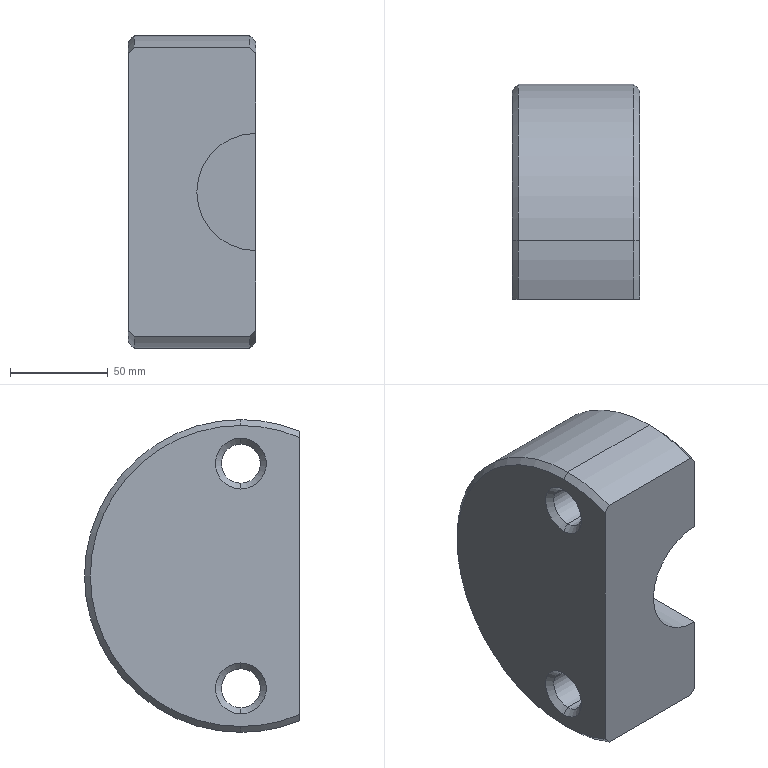Part | SolidWorks | features BaseBody 1 | 1 solid | 26 faces | box 65 x 110 x 160 mm | volume 821212 mm3 | cone 14 | cylinder 8 | plane 4 | commonest cylinder face diameters 20 x4 160 x3 60 x1
STEP:
#1=CARTESIAN_POINT('',(240.077,228.635,290.107));
#2=VERTEX_POINT('',#1);
#3=CARTESIAN_POINT('',(240.077,228.635,230.107));
#4=VERTEX_POINT('',#3);
#5=CARTESIAN_POINT('',(240.077,228.635,260.107));
#6=DIRECTION('',(0.,-1.,0.));
#7=DIRECTION('',(0.,0.,1.));
#8=AXIS2_PLACEMENT_3D('',#5,#6,#7);
#9=CIRCLE('',#8,30.);
#10=EDGE_CURVE('',#2,#4,#9,.T.);
#11=ORIENTED_EDGE('',*,*,#10,.F.);
#12=CARTESIAN_POINT('',(240.077,163.635,290.107));
#13=VERTEX_POINT('',#12);
#14=CARTESIAN_POINT('',(240.077,228.635,290.107));
#15=DIRECTION('',(0.,1.,0.));
#16=VECTOR('',#15,1000.);
#17=LINE('',#14,#16);
#18=EDGE_CURVE('',#13,#2,#17,.T.);
#19=ORIENTED_EDGE('',*,*,#18,.F.);
#20=CARTESIAN_POINT('',(240.077,163.635,230.107));
#21=VERTEX_POINT('',#20);
#22=CARTESIAN_POINT('',(240.077,163.635,260.107));
#23=DIRECTION('',(0.,-1.,0.));
#24=DIRECTION('',(0.,0.,1.));
#25=AXIS2_PLACEMENT_3D('',#22,#23,#24);
#26=CIRCLE('',#25,30.);
#27=EDGE_CURVE('',#13,#21,#26,.T.);
#28=ORIENTED_EDGE('',*,*,#27,.T.);
#29=CARTESIAN_POINT('',(240.077,228.635,230.107));
#30=DIRECTION('',(0.,-1.,0.));
#31=VECTOR('',#30,1000.);
#32=LINE('',#29,#31);
#33=EDGE_CURVE('',#4,#21,#32,.T.);
#34=ORIENTED_EDGE('',*,*,#33,.F.);
#35=EDGE_LOOP('',(#11,#19,#28,#34));
#36=FACE_OUTER_BOUND('',#35,.T.);
#37=CARTESIAN_POINT('',(240.077,228.635,260.107));
#38=DIRECTION('',(0.,-1.,0.));
#39=DIRECTION('',(0.,0.,-1.));
#40=AXIS2_PLACEMENT_3D('',#37,#38,#39);
#41=CYLINDRICAL_SURFACE('',#40,30.);
#42=ADVANCED_FACE('',(#36),#41,.F.);
#43=CARTESIAN_POINT('',(240.077,228.635,260.107));
#44=DIRECTION('',(0.,0.,1.));
#45=VECTOR('',#44,1000.);
#46=LINE('',#43,#45);
#47=EDGE_CURVE('',#4,#2,#46,.T.);
#48=ORIENTED_EDGE('',*,*,#47,.T.);
#49=ORIENTED_EDGE('',*,*,#10,.T.);
#50=EDGE_LOOP('',(#48,#49));
#51=FACE_OUTER_BOUND('',#50,.T.);
#52=CARTESIAN_POINT('',(240.077,228.635,260.107));
#53=DIRECTION('',(0.,-1.,0.));
#54=DIRECTION('',(0.,0.,-1.));
#55=AXIS2_PLACEMENT_3D('',#52,#53,#54);
#56=PLANE('',#55);
#57=ADVANCED_FACE('',(#51),#56,.T.);
#58=CARTESIAN_POINT('',(240.077,193.635,183.107));
#59=VERTEX_POINT('',#58);
#60=CARTESIAN_POINT('',(237.077,193.635,180.107));
#61=VERTEX_POINT('',#60);
#62=CARTESIAN_POINT('',(237.077,193.635,180.107));
#63=DIRECTION('',(-0.7071,0.,-0.7071));
#64=VECTOR('',#63,1000.);
#65=LINE('',#62,#64);
#66=EDGE_CURVE('',#59,#61,#65,.T.);
#67=ORIENTED_EDGE('',*,*,#66,.F.);
#68=CARTESIAN_POINT('',(240.077,163.635,189.191));
#69=VERTEX_POINT('',#68);
#70=CARTESIAN_POINT('',(240.077,193.635,260.107));
#71=DIRECTION('',(1.,0.,0.));
#72=DIRECTION('',(0.,0.,1.));
#73=AXIS2_PLACEMENT_3D('',#70,#71,#72);
#74=CIRCLE('',#73,77.);
#75=EDGE_CURVE('',#69,#59,#74,.T.);
#76=ORIENTED_EDGE('',*,*,#75,.F.);
#77=CARTESIAN_POINT('',(237.077,163.635,185.945));
#78=VERTEX_POINT('',#77);
#79=CARTESIAN_POINT('',(237.077,163.635,185.945));
#80=CARTESIAN_POINT('',(238.079,163.635,187.025));
#81=CARTESIAN_POINT('',(239.079,163.635,188.107));
#82=CARTESIAN_POINT('',(240.077,163.635,189.191));
#83=B_SPLINE_CURVE_WITH_KNOTS('',3,(#79,#80,#81,#82),.UNSPECIFIED.,.F.,.F.,(4,4),(0.,1.),.UNSPECIFIED.);
#84=EDGE_CURVE('',#78,#69,#83,.T.);
#85=ORIENTED_EDGE('',*,*,#84,.F.);
#86=CARTESIAN_POINT('',(237.077,193.635,260.107));
#87=DIRECTION('',(-1.,0.,0.));
#88=DIRECTION('',(0.,0.,1.));
#89=AXIS2_PLACEMENT_3D('',#86,#87,#88);
#90=CIRCLE('',#89,80.);
#91=EDGE_CURVE('',#61,#78,#90,.T.);
#92=ORIENTED_EDGE('',*,*,#91,.F.);
#93=EDGE_LOOP('',(#67,#76,#85,#92));
#94=FACE_OUTER_BOUND('',#93,.T.);
#95=CARTESIAN_POINT('',(237.077,193.635,260.107));
#96=DIRECTION('',(-1.,0.,0.));
#97=DIRECTION('',(0.,0.,-1.));
#98=AXIS2_PLACEMENT_3D('',#95,#96,#97);
#99=CONICAL_SURFACE('',#98,80.,0.7854);
#100=ADVANCED_FACE('',(#94),#99,.T.);
#101=CARTESIAN_POINT('',(175.077,193.635,337.107));
#102=VERTEX_POINT('',#101);
#103=CARTESIAN_POINT('',(178.077,193.635,340.107));
#104=VERTEX_POINT('',#103);
#105=CARTESIAN_POINT('',(175.077,193.635,337.107));
#106=DIRECTION('',(0.7071,0.,0.7071));
#107=VECTOR('',#106,1000.);
#108=LINE('',#105,#107);
#109=EDGE_CURVE('',#102,#104,#108,.T.);
#110=ORIENTED_EDGE('',*,*,#109,.F.);
#111=CARTESIAN_POINT('',(175.077,163.635,331.022));
#112=VERTEX_POINT('',#111);
#113=CARTESIAN_POINT('',(175.077,193.635,260.107));
#114=DIRECTION('',(-1.,0.,0.));
#115=DIRECTION('',(0.,0.,1.));
#116=AXIS2_PLACEMENT_3D('',#113,#114,#115);
#117=CIRCLE('',#116,77.);
#118=EDGE_CURVE('',#112,#102,#117,.T.);
#119=ORIENTED_EDGE('',*,*,#118,.F.);
#120=CARTESIAN_POINT('',(178.077,163.635,334.269));
#121=VERTEX_POINT('',#120);
#122=CARTESIAN_POINT('',(178.077,163.635,334.269));
#123=CARTESIAN_POINT('',(177.075,163.635,333.188));
#124=CARTESIAN_POINT('',(176.075,163.635,332.106));
#125=CARTESIAN_POINT('',(175.077,163.635,331.022));
#126=B_SPLINE_CURVE_WITH_KNOTS('',3,(#122,#123,#124,#125),.UNSPECIFIED.,.F.,.F.,(4,4),(0.,1.),.UNSPECIFIED.);
#127=EDGE_CURVE('',#121,#112,#126,.T.);
#128=ORIENTED_EDGE('',*,*,#127,.F.);
#129=CARTESIAN_POINT('',(178.077,193.635,260.107));
#130=DIRECTION('',(1.,0.,0.));
#131=DIRECTION('',(0.,0.,1.));
#132=AXIS2_PLACEMENT_3D('',#129,#130,#131);
#133=CIRCLE('',#132,80.);
#134=EDGE_CURVE('',#104,#121,#133,.T.);
#135=ORIENTED_EDGE('',*,*,#134,.F.);
#136=EDGE_LOOP('',(#110,#119,#128,#135));
#137=FACE_OUTER_BOUND('',#136,.T.);
#138=CARTESIAN_POINT('',(175.077,193.635,260.107));
#139=DIRECTION('',(1.,0.,0.));
#140=DIRECTION('',(0.,0.,1.));
#141=AXIS2_PLACEMENT_3D('',#138,#139,#140);
#142=CONICAL_SURFACE('',#141,77.,0.7854);
#143=ADVANCED_FACE('',(#137),#142,.T.);
#144=CARTESIAN_POINT('',(240.077,193.635,330.607));
#145=VERTEX_POINT('',#144);
#146=CARTESIAN_POINT('',(237.077,193.635,327.607));
#147=VERTEX_POINT('',#146);
#148=CARTESIAN_POINT('',(240.077,193.635,330.607));
#149=DIRECTION('',(-0.7071,0.,-0.7071));
#150=VECTOR('',#149,1000.);
#151=LINE('',#148,#150);
#152=EDGE_CURVE('',#145,#147,#151,.T.);
#153=ORIENTED_EDGE('',*,*,#152,.T.);
#154=CARTESIAN_POINT('',(237.077,193.635,307.607));
#155=VERTEX_POINT('',#154);
#156=CARTESIAN_POINT('',(237.077,193.635,317.607));
#157=DIRECTION('',(1.,0.,0.));
#158=DIRECTION('',(0.,0.,1.));
#159=AXIS2_PLACEMENT_3D('',#156,#157,#158);
#160=CIRCLE('',#159,10.);
#161=EDGE_CURVE('',#155,#147,#160,.T.);
#162=ORIENTED_EDGE('',*,*,#161,.F.);
#163=CARTESIAN_POINT('',(240.077,193.635,304.607));
#164=VERTEX_POINT('',#163);
#165=CARTESIAN_POINT('',(240.077,193.635,304.607));
#166=DIRECTION('',(-0.7071,0.,0.7071));
#167=VECTOR('',#166,1000.);
#168=LINE('',#165,#167);
#169=EDGE_CURVE('',#164,#155,#168,.T.);
#170=ORIENTED_EDGE('',*,*,#169,.F.);
#171=CARTESIAN_POINT('',(240.077,193.635,317.607));
#172=DIRECTION('',(-1.,0.,0.));
#173=DIRECTION('',(0.,0.,1.));
#174=AXIS2_PLACEMENT_3D('',#171,#172,#173);
#175=CIRCLE('',#174,13.);
#176=EDGE_CURVE('',#145,#164,#175,.T.);
#177=ORIENTED_EDGE('',*,*,#176,.F.);
#178=EDGE_LOOP('',(#153,#162,#170,#177));
#179=FACE_OUTER_BOUND('',#178,.T.);
#180=CARTESIAN_POINT('',(240.077,193.635,317.607));
#181=DIRECTION('',(1.,0.,0.));
#182=DIRECTION('',(0.,0.,1.));
#183=AXIS2_PLACEMENT_3D('',#180,#181,#182);
#184=CONICAL_SURFACE('',#183,13.,0.7854);
#185=ADVANCED_FACE('',(#179),#184,.F.);
#186=CARTESIAN_POINT('',(240.077,193.635,215.607));
#187=VERTEX_POINT('',#186);
#188=CARTESIAN_POINT('',(237.077,193.635,212.607));
#189=VERTEX_POINT('',#188);
#190=CARTESIAN_POINT('',(240.077,193.635,215.607));
#191=DIRECTION('',(-0.7071,0.,-0.7071));
#192=VECTOR('',#191,1000.);
#193=LINE('',#190,#192);
#194=EDGE_CURVE('',#187,#189,#193,.T.);
#195=ORIENTED_EDGE('',*,*,#194,.T.);
#196=CARTESIAN_POINT('',(237.077,193.635,192.607));
#197=VERTEX_POINT('',#196);
#198=CARTESIAN_POINT('',(237.077,193.635,202.607));
#199=DIRECTION('',(1.,0.,0.));
#200=DIRECTION('',(0.,0.,1.));
#201=AXIS2_PLACEMENT_3D('',#198,#199,#200);
#202=CIRCLE('',#201,10.);
#203=EDGE_CURVE('',#197,#189,#202,.T.);
#204=ORIENTED_EDGE('',*,*,#203,.F.);
#205=CARTESIAN_POINT('',(240.077,193.635,189.607));
#206=VERTEX_POINT('',#205);
#207=CARTESIAN_POINT('',(240.077,193.635,189.607));
#208=DIRECTION('',(-0.7071,0.,0.7071));
#209=VECTOR('',#208,1000.);
#210=LINE('',#207,#209);
#211=EDGE_CURVE('',#206,#197,#210,.T.);
#212=ORIENTED_EDGE('',*,*,#211,.F.);
#213=CARTESIAN_POINT('',(240.077,193.635,202.607));
#214=DIRECTION('',(-1.,0.,0.));
#215=DIRECTION('',(0.,0.,1.));
#216=AXIS2_PLACEMENT_3D('',#213,#214,#215);
#217=CIRCLE('',#216,13.);
#218=EDGE_CURVE('',#187,#206,#217,.T.);
#219=ORIENTED_EDGE('',*,*,#218,.F.);
#220=EDGE_LOOP('',(#195,#204,#212,#219));
#221=FACE_OUTER_BOUND('',#220,.T.);
#222=CARTESIAN_POINT('',(240.077,193.635,202.607));
#223=DIRECTION('',(1.,0.,0.));
#224=DIRECTION('',(0.,0.,1.));
#225=AXIS2_PLACEMENT_3D('',#222,#223,#224);
#226=CONICAL_SURFACE('',#225,13.,0.7854);
#227=ADVANCED_FACE('',(#221),#226,.F.);
#228=CARTESIAN_POINT('',(175.077,193.635,189.607));
#229=VERTEX_POINT('',#228);
#230=CARTESIAN_POINT('',(178.077,193.635,192.607));
#231=VERTEX_POINT('',#230);
#232=CARTESIAN_POINT('',(178.077,193.635,192.607));
#233=DIRECTION('',(0.7071,0.,0.7071));
#234=VECTOR('',#233,1000.);
#235=LINE('',#232,#234);
#236=EDGE_CURVE('',#229,#231,#235,.T.);
#237=ORIENTED_EDGE('',*,*,#236,.T.);
#238=CARTESIAN_POINT('',(178.077,193.635,212.607));
#239=VERTEX_POINT('',#238);
#240=CARTESIAN_POINT('',(178.077,193.635,202.607));
#241=DIRECTION('',(-1.,0.,0.));
#242=DIRECTION('',(0.,0.,1.));
#243=AXIS2_PLACEMENT_3D('',#240,#241,#242);
#244=CIRCLE('',#243,10.);
#245=EDGE_CURVE('',#239,#231,#244,.T.);
#246=ORIENTED_EDGE('',*,*,#245,.F.);
#247=CARTESIAN_POINT('',(175.077,193.635,215.607));
#248=VERTEX_POINT('',#247);
#249=CARTESIAN_POINT('',(178.077,193.635,212.607));
#250=DIRECTION('',(0.7071,0.,-0.7071));
#251=VECTOR('',#250,1000.);
#252=LINE('',#249,#251);
#253=EDGE_CURVE('',#248,#239,#252,.T.);
#254=ORIENTED_EDGE('',*,*,#253,.F.);
#255=CARTESIAN_POINT('',(175.077,193.635,202.607));
#256=DIRECTION('',(1.,0.,0.));
#257=DIRECTION('',(0.,0.,1.));
#258=AXIS2_PLACEMENT_3D('',#255,#256,#257);
#259=CIRCLE('',#258,13.);
#260=EDGE_CURVE('',#229,#248,#259,.T.);
#261=ORIENTED_EDGE('',*,*,#260,.F.);
#262=EDGE_LOOP('',(#237,#246,#254,#261));
#263=FACE_OUTER_BOUND('',#262,.T.);
#264=CARTESIAN_POINT('',(178.077,193.635,202.607));
#265=DIRECTION('',(-1.,0.,0.));
#266=DIRECTION('',(0.,0.,-1.));
#267=AXIS2_PLACEMENT_3D('',#264,#265,#266);
#268=CONICAL_SURFACE('',#267,10.,0.7854);
#269=ADVANCED_FACE('',(#263),#268,.F.);
#270=CARTESIAN_POINT('',(175.077,193.635,304.607));
#271=VERTEX_POINT('',#270);
#272=CARTESIAN_POINT('',(178.077,193.635,307.607));
#273=VERTEX_POINT('',#272);
#274=CARTESIAN_POINT('',(178.077,193.635,307.607));
#275=DIRECTION('',(0.7071,0.,0.7071));
#276=VECTOR('',#275,1000.);
#277=LINE('',#274,#276);
#278=EDGE_CURVE('',#271,#273,#277,.T.);
#279=ORIENTED_EDGE('',*,*,#278,.T.);
#280=CARTESIAN_POINT('',(178.077,193.635,327.607));
#281=VERTEX_POINT('',#280);
#282=CARTESIAN_POINT('',(178.077,193.635,317.607));
#283=DIRECTION('',(-1.,0.,0.));
#284=DIRECTION('',(0.,0.,1.));
#285=AXIS2_PLACEMENT_3D('',#282,#283,#284);
#286=CIRCLE('',#285,10.);
#287=EDGE_CURVE('',#281,#273,#286,.T.);
#288=ORIENTED_EDGE('',*,*,#287,.F.);
#289=CARTESIAN_POINT('',(175.077,193.635,330.607));
#290=VERTEX_POINT('',#289);
#291=CARTESIAN_POINT('',(178.077,193.635,327.607));
#292=DIRECTION('',(0.7071,0.,-0.7071));
#293=VECTOR('',#292,1000.);
#294=LINE('',#291,#293);
#295=EDGE_CURVE('',#290,#281,#294,.T.);
#296=ORIENTED_EDGE('',*,*,#295,.F.);
#297=CARTESIAN_POINT('',(175.077,193.635,317.607));
#298=DIRECTION('',(1.,0.,0.));
#299=DIRECTION('',(0.,0.,1.));
#300=AXIS2_PLACEMENT_3D('',#297,#298,#299);
#301=CIRCLE('',#300,13.);
#302=EDGE_CURVE('',#271,#290,#301,.T.);
#303=ORIENTED_EDGE('',*,*,#302,.F.);
#304=EDGE_LOOP('',(#279,#288,#296,#303));
#305=FACE_OUTER_BOUND('',#304,.T.);
#306=CARTESIAN_POINT('',(178.077,193.635,317.607));
#307=DIRECTION('',(-1.,0.,0.));
#308=DIRECTION('',(0.,0.,-1.));
#309=AXIS2_PLACEMENT_3D('',#306,#307,#308);
#310=CONICAL_SURFACE('',#309,10.,0.7854);
#311=ADVANCED_FACE('',(#305),#310,.F.);
#312=CARTESIAN_POINT('',(175.077,193.635,327.607));
#313=DIRECTION('',(-1.,0.,0.));
#314=VECTOR('',#313,1000.);
#315=LINE('',#312,#314);
#316=EDGE_CURVE('',#147,#281,#315,.T.);
#317=ORIENTED_EDGE('',*,*,#316,.T.);
#318=ORIENTED_EDGE('',*,*,#287,.T.);
#319=CARTESIAN_POINT('',(175.077,193.635,307.607));
#320=DIRECTION('',(-1.,0.,0.));
#321=VECTOR('',#320,1000.);
#322=LINE('',#319,#321);
#323=EDGE_CURVE('',#155,#273,#322,.T.);
#324=ORIENTED_EDGE('',*,*,#323,.F.);
#325=ORIENTED_EDGE('',*,*,#161,.T.);
#326=EDGE_LOOP('',(#317,#318,#324,#325));
#327=FACE_OUTER_BOUND('',#326,.T.);
#328=CARTESIAN_POINT('',(175.077,193.635,317.607));
#329=DIRECTION('',(1.,0.,0.));
#330=DIRECTION('',(0.,0.,1.));
#331=AXIS2_PLACEMENT_3D('',#328,#329,#330);
#332=CYLINDRICAL_SURFACE('',#331,10.);
#333=ADVANCED_FACE('',(#327),#332,.F.);
#334=CARTESIAN_POINT('',(175.077,193.635,212.607));
#335=DIRECTION('',(-1.,0.,0.));
#336=VECTOR('',#335,1000.);
#337=LINE('',#334,#336);
#338=EDGE_CURVE('',#189,#239,#337,.T.);
#339=ORIENTED_EDGE('',*,*,#338,.T.);
#340=ORIENTED_EDGE('',*,*,#245,.T.);
#341=CARTESIAN_POINT('',(175.077,193.635,192.607));
#342=DIRECTION('',(-1.,0.,0.));
#343=VECTOR('',#342,1000.);
#344=LINE('',#341,#343);
#345=EDGE_CURVE('',#197,#231,#344,.T.);
#346=ORIENTED_EDGE('',*,*,#345,.F.);
#347=ORIENTED_EDGE('',*,*,#203,.T.);
#348=EDGE_LOOP('',(#339,#340,#346,#347));
#349=FACE_OUTER_BOUND('',#348,.T.);
#350=CARTESIAN_POINT('',(175.077,193.635,202.607));
#351=DIRECTION('',(1.,0.,0.));
#352=DIRECTION('',(0.,0.,1.));
#353=AXIS2_PLACEMENT_3D('',#350,#351,#352);
#354=CYLINDRICAL_SURFACE('',#353,10.);
#355=ADVANCED_FACE('',(#349),#354,.F.);
#356=CARTESIAN_POINT('',(240.077,163.635,260.107));
#357=DIRECTION('',(0.,0.,1.));
#358=VECTOR('',#357,1000.);
#359=LINE('',#356,#358);
#360=EDGE_CURVE('',#69,#21,#359,.T.);
#361=ORIENTED_EDGE('',*,*,#360,.T.);
#362=ORIENTED_EDGE('',*,*,#27,.F.);
#363=CARTESIAN_POINT('',(240.077,163.635,331.022));
#364=VERTEX_POINT('',#363);
#365=CARTESIAN_POINT('',(240.077,163.635,260.107));
#366=DIRECTION('',(0.,0.,1.));
#367=VECTOR('',#366,1000.);
#368=LINE('',#365,#367);
#369=EDGE_CURVE('',#13,#364,#368,.T.);
#370=ORIENTED_EDGE('',*,*,#369,.T.);
#371=CARTESIAN_POINT('',(237.077,163.635,334.269));
#372=VERTEX_POINT('',#371);
#373=CARTESIAN_POINT('',(240.077,163.635,331.022));
#374=CARTESIAN_POINT('',(239.079,163.635,332.106));
#375=CARTESIAN_POINT('',(238.079,163.635,333.188));
#376=CARTESIAN_POINT('',(237.077,163.635,334.269));
#377=B_SPLINE_CURVE_WITH_KNOTS('',3,(#373,#374,#375,#376),.UNSPECIFIED.,.F.,.F.,(4,4),(0.,1.),.UNSPECIFIED.);
#378=EDGE_CURVE('',#364,#372,#377,.T.);
#379=ORIENTED_EDGE('',*,*,#378,.T.);
#380=CARTESIAN_POINT('',(175.077,163.635,334.269));
#381=DIRECTION('',(1.,0.,0.));
#382=VECTOR('',#381,1000.);
#383=LINE('',#380,#382);
#384=EDGE_CURVE('',#121,#372,#383,.T.);
#385=ORIENTED_EDGE('',*,*,#384,.F.);
#386=ORIENTED_EDGE('',*,*,#127,.T.);
#387=CARTESIAN_POINT('',(175.077,163.635,189.191));
#388=VERTEX_POINT('',#387);
#389=CARTESIAN_POINT('',(175.077,163.635,260.107));
#390=DIRECTION('',(0.,0.,1.));
#391=VECTOR('',#390,1000.);
#392=LINE('',#389,#391);
#393=EDGE_CURVE('',#388,#112,#392,.T.);
#394=ORIENTED_EDGE('',*,*,#393,.F.);
#395=CARTESIAN_POINT('',(178.077,163.635,185.945));
#396=VERTEX_POINT('',#395);
#397=CARTESIAN_POINT('',(175.077,163.635,189.191));
#398=CARTESIAN_POINT('',(176.075,163.635,188.107));
#399=CARTESIAN_POINT('',(177.075,163.635,187.025));
#400=CARTESIAN_POINT('',(178.077,163.635,185.945));
#401=B_SPLINE_CURVE_WITH_KNOTS('',3,(#397,#398,#399,#400),.UNSPECIFIED.,.F.,.F.,(4,4),(0.,1.),.UNSPECIFIED.);
#402=EDGE_CURVE('',#388,#396,#401,.T.);
#403=ORIENTED_EDGE('',*,*,#402,.T.);
#404=CARTESIAN_POINT('',(175.077,163.635,185.945));
#405=DIRECTION('',(1.,0.,0.));
#406=VECTOR('',#405,1000.);
#407=LINE('',#404,#406);
#408=EDGE_CURVE('',#396,#78,#407,.T.);
#409=ORIENTED_EDGE('',*,*,#408,.T.);
#410=ORIENTED_EDGE('',*,*,#84,.T.);
#411=EDGE_LOOP('',(#361,#362,#370,#379,#385,#386,#394,#403,#409,#410));
#412=FACE_OUTER_BOUND('',#411,.T.);
#413=CARTESIAN_POINT('',(175.077,163.635,260.107));
#414=DIRECTION('',(0.,1.,0.));
#415=DIRECTION('',(1.,0.,0.));
#416=AXIS2_PLACEMENT_3D('',#413,#414,#415);
#417=PLANE('',#416);
#418=ADVANCED_FACE('',(#412),#417,.F.);
#419=CARTESIAN_POINT('',(237.077,193.635,340.107));
#420=VERTEX_POINT('',#419);
#421=CARTESIAN_POINT('',(175.077,193.635,340.107));
#422=DIRECTION('',(1.,0.,0.));
#423=VECTOR('',#422,1000.);
#424=LINE('',#421,#423);
#425=EDGE_CURVE('',#104,#420,#424,.T.);
#426=ORIENTED_EDGE('',*,*,#425,.F.);
#427=ORIENTED_EDGE('',*,*,#134,.T.);
#428=ORIENTED_EDGE('',*,*,#384,.T.);
#429=CARTESIAN_POINT('',(237.077,193.635,260.107));
#430=DIRECTION('',(-1.,0.,0.));
#431=DIRECTION('',(0.,0.,1.));
#432=AXIS2_PLACEMENT_3D('',#429,#430,#431);
#433=CIRCLE('',#432,80.);
#434=EDGE_CURVE('',#372,#420,#433,.T.);
#435=ORIENTED_EDGE('',*,*,#434,.T.);
#436=EDGE_LOOP('',(#426,#427,#428,#435));
#437=FACE_OUTER_BOUND('',#436,.T.);
#438=CARTESIAN_POINT('',(175.077,193.635,260.107));
#439=DIRECTION('',(1.,0.,0.));
#440=DIRECTION('',(0.,0.,1.));
#441=AXIS2_PLACEMENT_3D('',#438,#439,#440);
#442=CYLINDRICAL_SURFACE('',#441,80.);
#443=ADVANCED_FACE('',(#437),#442,.T.);
#444=CARTESIAN_POINT('',(240.077,193.635,317.607));
#445=DIRECTION('',(-1.,0.,0.));
#446=DIRECTION('',(0.,0.,1.));
#447=AXIS2_PLACEMENT_3D('',#444,#445,#446);
#448=CIRCLE('',#447,13.);
#449=EDGE_CURVE('',#164,#145,#448,.T.);
#450=ORIENTED_EDGE('',*,*,#449,.T.);
#451=ORIENTED_EDGE('',*,*,#176,.T.);
#452=EDGE_LOOP('',(#450,#451));
#453=FACE_BOUND('',#452,.T.);
#454=CARTESIAN_POINT('',(240.077,193.635,202.607));
#455=DIRECTION('',(-1.,0.,0.));
#456=DIRECTION('',(0.,0.,1.));
#457=AXIS2_PLACEMENT_3D('',#454,#455,#456);
#458=CIRCLE('',#457,13.);
#459=EDGE_CURVE('',#206,#187,#458,.T.);
#460=ORIENTED_EDGE('',*,*,#459,.T.);
#461=ORIENTED_EDGE('',*,*,#218,.T.);
#462=EDGE_LOOP('',(#460,#461));
#463=FACE_BOUND('',#462,.T.);
#464=ORIENTED_EDGE('',*,*,#47,.F.);
#465=ORIENTED_EDGE('',*,*,#33,.T.);
#466=ORIENTED_EDGE('',*,*,#360,.F.);
#467=ORIENTED_EDGE('',*,*,#75,.T.);
#468=CARTESIAN_POINT('',(240.077,193.635,337.107));
#469=VERTEX_POINT('',#468);
#470=CARTESIAN_POINT('',(240.077,193.635,260.107));
#471=DIRECTION('',(1.,0.,0.));
#472=DIRECTION('',(0.,0.,1.));
#473=AXIS2_PLACEMENT_3D('',#470,#471,#472);
#474=CIRCLE('',#473,77.);
#475=EDGE_CURVE('',#59,#469,#474,.T.);
#476=ORIENTED_EDGE('',*,*,#475,.T.);
#477=CARTESIAN_POINT('',(240.077,193.635,260.107));
#478=DIRECTION('',(1.,0.,0.));
#479=DIRECTION('',(0.,0.,1.));
#480=AXIS2_PLACEMENT_3D('',#477,#478,#479);
#481=CIRCLE('',#480,77.);
#482=EDGE_CURVE('',#469,#364,#481,.T.);
#483=ORIENTED_EDGE('',*,*,#482,.T.);
#484=ORIENTED_EDGE('',*,*,#369,.F.);
#485=ORIENTED_EDGE('',*,*,#18,.T.);
#486=EDGE_LOOP('',(#464,#465,#466,#467,#476,#483,#484,#485));
#487=FACE_OUTER_BOUND('',#486,.T.);
#488=CARTESIAN_POINT('',(240.077,193.635,260.107));
#489=DIRECTION('',(-1.,0.,0.));
#490=DIRECTION('',(0.,0.,1.));
#491=AXIS2_PLACEMENT_3D('',#488,#489,#490);
#492=PLANE('',#491);
#493=ADVANCED_FACE('',(#453,#463,#487),#492,.F.);
#494=CARTESIAN_POINT('',(175.077,193.635,202.607));
#495=DIRECTION('',(1.,0.,0.));
#496=DIRECTION('',(0.,0.,1.));
#497=AXIS2_PLACEMENT_3D('',#494,#495,#496);
#498=CIRCLE('',#497,13.);
#499=EDGE_CURVE('',#248,#229,#498,.T.);
#500=ORIENTED_EDGE('',*,*,#499,.T.);
#501=ORIENTED_EDGE('',*,*,#260,.T.);
#502=EDGE_LOOP('',(#500,#501));
#503=FACE_BOUND('',#502,.T.);
#504=CARTESIAN_POINT('',(175.077,193.635,317.607));
#505=DIRECTION('',(1.,0.,0.));
#506=DIRECTION('',(0.,0.,1.));
#507=AXIS2_PLACEMENT_3D('',#504,#505,#506);
#508=CIRCLE('',#507,13.);
#509=EDGE_CURVE('',#290,#271,#508,.T.);
#510=ORIENTED_EDGE('',*,*,#509,.T.);
#511=ORIENTED_EDGE('',*,*,#302,.T.);
#512=EDGE_LOOP('',(#510,#511));
#513=FACE_BOUND('',#512,.T.);
#514=ORIENTED_EDGE('',*,*,#393,.T.);
#515=ORIENTED_EDGE('',*,*,#118,.T.);
#516=CARTESIAN_POINT('',(175.077,193.635,183.107));
#517=VERTEX_POINT('',#516);
#518=CARTESIAN_POINT('',(175.077,193.635,260.107));
#519=DIRECTION('',(-1.,0.,0.));
#520=DIRECTION('',(0.,0.,1.));
#521=AXIS2_PLACEMENT_3D('',#518,#519,#520);
#522=CIRCLE('',#521,77.);
#523=EDGE_CURVE('',#102,#517,#522,.T.);
#524=ORIENTED_EDGE('',*,*,#523,.T.);
#525=CARTESIAN_POINT('',(175.077,193.635,260.107));
#526=DIRECTION('',(-1.,0.,0.));
#527=DIRECTION('',(0.,0.,1.));
#528=AXIS2_PLACEMENT_3D('',#525,#526,#527);
#529=CIRCLE('',#528,77.);
#530=EDGE_CURVE('',#517,#388,#529,.T.);
#531=ORIENTED_EDGE('',*,*,#530,.T.);
#532=EDGE_LOOP('',(#514,#515,#524,#531));
#533=FACE_OUTER_BOUND('',#532,.T.);
#534=CARTESIAN_POINT('',(175.077,193.635,260.107));
#535=DIRECTION('',(-1.,0.,0.));
#536=DIRECTION('',(0.,0.,1.));
#537=AXIS2_PLACEMENT_3D('',#534,#535,#536);
#538=PLANE('',#537);
#539=ADVANCED_FACE('',(#503,#513,#533),#538,.T.);
#540=CARTESIAN_POINT('',(178.077,193.635,180.107));
#541=VERTEX_POINT('',#540);
#542=CARTESIAN_POINT('',(178.077,193.635,260.107));
#543=DIRECTION('',(1.,0.,0.));
#544=DIRECTION('',(0.,0.,1.));
#545=AXIS2_PLACEMENT_3D('',#542,#543,#544);
#546=CIRCLE('',#545,80.);
#547=EDGE_CURVE('',#396,#541,#546,.T.);
#548=ORIENTED_EDGE('',*,*,#547,.T.);
#549=CARTESIAN_POINT('',(175.077,193.635,180.107));
#550=DIRECTION('',(1.,0.,0.));
#551=VECTOR('',#550,1000.);
#552=LINE('',#549,#551);
#553=EDGE_CURVE('',#541,#61,#552,.T.);
#554=ORIENTED_EDGE('',*,*,#553,.T.);
#555=ORIENTED_EDGE('',*,*,#91,.T.);
#556=ORIENTED_EDGE('',*,*,#408,.F.);
#557=EDGE_LOOP('',(#548,#554,#555,#556));
#558=FACE_OUTER_BOUND('',#557,.T.);
#559=CARTESIAN_POINT('',(175.077,193.635,260.107));
#560=DIRECTION('',(1.,0.,0.));
#561=DIRECTION('',(0.,0.,1.));
#562=AXIS2_PLACEMENT_3D('',#559,#560,#561);
#563=CYLINDRICAL_SURFACE('',#562,80.);
#564=ADVANCED_FACE('',(#558),#563,.T.);
#565=CARTESIAN_POINT('',(178.077,193.635,260.107));
#566=DIRECTION('',(1.,0.,0.));
#567=DIRECTION('',(0.,0.,1.));
#568=AXIS2_PLACEMENT_3D('',#565,#566,#567);
#569=CIRCLE('',#568,80.);
#570=EDGE_CURVE('',#541,#104,#569,.T.);
#571=ORIENTED_EDGE('',*,*,#570,.T.);
#572=ORIENTED_EDGE('',*,*,#425,.T.);
#573=CARTESIAN_POINT('',(237.077,193.635,260.107));
#574=DIRECTION('',(-1.,0.,0.));
#575=DIRECTION('',(0.,0.,1.));
#576=AXIS2_PLACEMENT_3D('',#573,#574,#575);
#577=CIRCLE('',#576,80.);
#578=EDGE_CURVE('',#420,#61,#577,.T.);
#579=ORIENTED_EDGE('',*,*,#578,.T.);
#580=ORIENTED_EDGE('',*,*,#553,.F.);
#581=EDGE_LOOP('',(#571,#572,#579,#580));
#582=FACE_OUTER_BOUND('',#581,.T.);
#583=CARTESIAN_POINT('',(175.077,193.635,260.107));
#584=DIRECTION('',(1.,0.,0.));
#585=DIRECTION('',(0.,0.,1.));
#586=AXIS2_PLACEMENT_3D('',#583,#584,#585);
#587=CYLINDRICAL_SURFACE('',#586,80.);
#588=ADVANCED_FACE('',(#582),#587,.T.);
#589=CARTESIAN_POINT('',(178.077,193.635,202.607));
#590=DIRECTION('',(-1.,0.,0.));
#591=DIRECTION('',(0.,0.,1.));
#592=AXIS2_PLACEMENT_3D('',#589,#590,#591);
#593=CIRCLE('',#592,10.);
#594=EDGE_CURVE('',#231,#239,#593,.T.);
#595=ORIENTED_EDGE('',*,*,#594,.T.);
#596=ORIENTED_EDGE('',*,*,#338,.F.);
#597=CARTESIAN_POINT('',(237.077,193.635,202.607));
#598=DIRECTION('',(1.,0.,0.));
#599=DIRECTION('',(0.,0.,1.));
#600=AXIS2_PLACEMENT_3D('',#597,#598,#599);
#601=CIRCLE('',#600,10.);
#602=EDGE_CURVE('',#189,#197,#601,.T.);
#603=ORIENTED_EDGE('',*,*,#602,.T.);
#604=ORIENTED_EDGE('',*,*,#345,.T.);
#605=EDGE_LOOP('',(#595,#596,#603,#604));
#606=FACE_OUTER_BOUND('',#605,.T.);
#607=CARTESIAN_POINT('',(175.077,193.635,202.607));
#608=DIRECTION('',(1.,0.,0.));
#609=DIRECTION('',(0.,0.,1.));
#610=AXIS2_PLACEMENT_3D('',#607,#608,#609);
#611=CYLINDRICAL_SURFACE('',#610,10.);
#612=ADVANCED_FACE('',(#606),#611,.F.);
#613=CARTESIAN_POINT('',(178.077,193.635,317.607));
#614=DIRECTION('',(-1.,0.,0.));
#615=DIRECTION('',(0.,0.,1.));
#616=AXIS2_PLACEMENT_3D('',#613,#614,#615);
#617=CIRCLE('',#616,10.);
#618=EDGE_CURVE('',#273,#281,#617,.T.);
#619=ORIENTED_EDGE('',*,*,#618,.T.);
#620=ORIENTED_EDGE('',*,*,#316,.F.);
#621=CARTESIAN_POINT('',(237.077,193.635,317.607));
#622=DIRECTION('',(1.,0.,0.));
#623=DIRECTION('',(0.,0.,1.));
#624=AXIS2_PLACEMENT_3D('',#621,#622,#623);
#625=CIRCLE('',#624,10.);
#626=EDGE_CURVE('',#147,#155,#625,.T.);
#627=ORIENTED_EDGE('',*,*,#626,.T.);
#628=ORIENTED_EDGE('',*,*,#323,.T.);
#629=EDGE_LOOP('',(#619,#620,#627,#628));
#630=FACE_OUTER_BOUND('',#629,.T.);
#631=CARTESIAN_POINT('',(175.077,193.635,317.607));
#632=DIRECTION('',(1.,0.,0.));
#633=DIRECTION('',(0.,0.,1.));
#634=AXIS2_PLACEMENT_3D('',#631,#632,#633);
#635=CYLINDRICAL_SURFACE('',#634,10.);
#636=ADVANCED_FACE('',(#630),#635,.F.);
#637=ORIENTED_EDGE('',*,*,#618,.F.);
#638=ORIENTED_EDGE('',*,*,#278,.F.);
#639=ORIENTED_EDGE('',*,*,#509,.F.);
#640=ORIENTED_EDGE('',*,*,#295,.T.);
#641=EDGE_LOOP('',(#637,#638,#639,#640));
#642=FACE_OUTER_BOUND('',#641,.T.);
#643=CARTESIAN_POINT('',(178.077,193.635,317.607));
#644=DIRECTION('',(-1.,0.,0.));
#645=DIRECTION('',(0.,0.,-1.));
#646=AXIS2_PLACEMENT_3D('',#643,#644,#645);
#647=CONICAL_SURFACE('',#646,10.,0.7854);
#648=ADVANCED_FACE('',(#642),#647,.F.);
#649=ORIENTED_EDGE('',*,*,#594,.F.);
#650=ORIENTED_EDGE('',*,*,#236,.F.);
#651=ORIENTED_EDGE('',*,*,#499,.F.);
#652=ORIENTED_EDGE('',*,*,#253,.T.);
#653=EDGE_LOOP('',(#649,#650,#651,#652));
#654=FACE_OUTER_BOUND('',#653,.T.);
#655=CARTESIAN_POINT('',(178.077,193.635,202.607));
#656=DIRECTION('',(-1.,0.,0.));
#657=DIRECTION('',(0.,0.,-1.));
#658=AXIS2_PLACEMENT_3D('',#655,#656,#657);
#659=CONICAL_SURFACE('',#658,10.,0.7854);
#660=ADVANCED_FACE('',(#654),#659,.F.);
#661=ORIENTED_EDGE('',*,*,#602,.F.);
#662=ORIENTED_EDGE('',*,*,#194,.F.);
#663=ORIENTED_EDGE('',*,*,#459,.F.);
#664=ORIENTED_EDGE('',*,*,#211,.T.);
#665=EDGE_LOOP('',(#661,#662,#663,#664));
#666=FACE_OUTER_BOUND('',#665,.T.);
#667=CARTESIAN_POINT('',(240.077,193.635,202.607));
#668=DIRECTION('',(1.,0.,0.));
#669=DIRECTION('',(0.,0.,1.));
#670=AXIS2_PLACEMENT_3D('',#667,#668,#669);
#671=CONICAL_SURFACE('',#670,13.,0.7854);
#672=ADVANCED_FACE('',(#666),#671,.F.);
#673=ORIENTED_EDGE('',*,*,#626,.F.);
#674=ORIENTED_EDGE('',*,*,#152,.F.);
#675=ORIENTED_EDGE('',*,*,#449,.F.);
#676=ORIENTED_EDGE('',*,*,#169,.T.);
#677=EDGE_LOOP('',(#673,#674,#675,#676));
#678=FACE_OUTER_BOUND('',#677,.T.);
#679=CARTESIAN_POINT('',(240.077,193.635,317.607));
#680=DIRECTION('',(1.,0.,0.));
#681=DIRECTION('',(0.,0.,1.));
#682=AXIS2_PLACEMENT_3D('',#679,#680,#681);
#683=CONICAL_SURFACE('',#682,13.,0.7854);
#684=ADVANCED_FACE('',(#678),#683,.F.);
#685=ORIENTED_EDGE('',*,*,#530,.F.);
#686=CARTESIAN_POINT('',(175.077,193.635,183.107));
#687=DIRECTION('',(0.7071,0.,-0.7071));
#688=VECTOR('',#687,1000.);
#689=LINE('',#686,#688);
#690=EDGE_CURVE('',#517,#541,#689,.T.);
#691=ORIENTED_EDGE('',*,*,#690,.T.);
#692=ORIENTED_EDGE('',*,*,#547,.F.);
#693=ORIENTED_EDGE('',*,*,#402,.F.);
#694=EDGE_LOOP('',(#685,#691,#692,#693));
#695=FACE_OUTER_BOUND('',#694,.T.);
#696=CARTESIAN_POINT('',(175.077,193.635,260.107));
#697=DIRECTION('',(1.,0.,0.));
#698=DIRECTION('',(0.,0.,1.));
#699=AXIS2_PLACEMENT_3D('',#696,#697,#698);
#700=CONICAL_SURFACE('',#699,77.,0.7854);
#701=ADVANCED_FACE('',(#695),#700,.T.);
#702=ORIENTED_EDGE('',*,*,#523,.F.);
#703=ORIENTED_EDGE('',*,*,#109,.T.);
#704=ORIENTED_EDGE('',*,*,#570,.F.);
#705=ORIENTED_EDGE('',*,*,#690,.F.);
#706=EDGE_LOOP('',(#702,#703,#704,#705));
#707=FACE_OUTER_BOUND('',#706,.T.);
#708=CARTESIAN_POINT('',(175.077,193.635,260.107));
#709=DIRECTION('',(1.,0.,0.));
#710=DIRECTION('',(0.,0.,1.));
#711=AXIS2_PLACEMENT_3D('',#708,#709,#710);
#712=CONICAL_SURFACE('',#711,77.,0.7854);
#713=ADVANCED_FACE('',(#707),#712,.T.);
#714=ORIENTED_EDGE('',*,*,#482,.F.);
#715=CARTESIAN_POINT('',(237.077,193.635,340.107));
#716=DIRECTION('',(-0.7071,0.,0.7071));
#717=VECTOR('',#716,1000.);
#718=LINE('',#715,#717);
#719=EDGE_CURVE('',#469,#420,#718,.T.);
#720=ORIENTED_EDGE('',*,*,#719,.T.);
#721=ORIENTED_EDGE('',*,*,#434,.F.);
#722=ORIENTED_EDGE('',*,*,#378,.F.);
#723=EDGE_LOOP('',(#714,#720,#721,#722));
#724=FACE_OUTER_BOUND('',#723,.T.);
#725=CARTESIAN_POINT('',(237.077,193.635,260.107));
#726=DIRECTION('',(-1.,0.,0.));
#727=DIRECTION('',(0.,0.,-1.));
#728=AXIS2_PLACEMENT_3D('',#725,#726,#727);
#729=CONICAL_SURFACE('',#728,80.,0.7854);
#730=ADVANCED_FACE('',(#724),#729,.T.);
#731=ORIENTED_EDGE('',*,*,#475,.F.);
#732=ORIENTED_EDGE('',*,*,#66,.T.);
#733=ORIENTED_EDGE('',*,*,#578,.F.);
#734=ORIENTED_EDGE('',*,*,#719,.F.);
#735=EDGE_LOOP('',(#731,#732,#733,#734));
#736=FACE_OUTER_BOUND('',#735,.T.);
#737=CARTESIAN_POINT('',(237.077,193.635,260.107));
#738=DIRECTION('',(-1.,0.,0.));
#739=DIRECTION('',(0.,0.,-1.));
#740=AXIS2_PLACEMENT_3D('',#737,#738,#739);
#741=CONICAL_SURFACE('',#740,80.,0.7854);
#742=ADVANCED_FACE('',(#736),#741,.T.);
#743=CLOSED_SHELL('',(#42,#57,#100,#143,#185,#227,#269,#311,#333,#355,#418,#443,#493,#539,#564,#588,#612,#636,#648,#660,#672,#684,#701,#713,#730,#742));
#744=MANIFOLD_SOLID_BREP('',#743);
#745=CARTESIAN_POINT('',(0.,0.,0.));
#746=DIRECTION('',(0.,0.,1.));
#747=DIRECTION('',(1.,0.,0.));
#748=AXIS2_PLACEMENT_3D('',#745,#746,#747);
#749=(LENGTH_UNIT()NAMED_UNIT(*)SI_UNIT(.MILLI.,.METRE.));
#750=UNCERTAINTY_MEASURE_WITH_UNIT(LENGTH_MEASURE(0.00001),#749,'','');
#751=(NAMED_UNIT(*)PLANE_ANGLE_UNIT()SI_UNIT($,.RADIAN.));
#752=(NAMED_UNIT(*)SI_UNIT($,.STERADIAN.)SOLID_ANGLE_UNIT());
#753=(GEOMETRIC_REPRESENTATION_CONTEXT(3)GLOBAL_UNCERTAINTY_ASSIGNED_CONTEXT((#750))GLOBAL_UNIT_ASSIGNED_CONTEXT((#749,#751,#752))REPRESENTATION_CONTEXT('',''));
#754=ADVANCED_BREP_SHAPE_REPRESENTATION('',(#744,#748),#753);